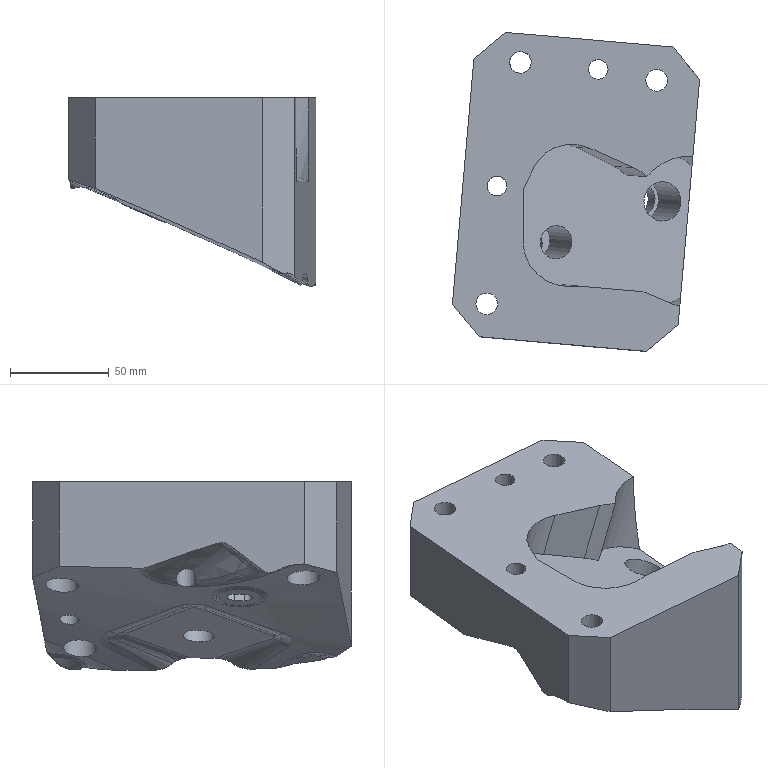Part | NX | features solid 2 | 1 solid | 91 faces | box 125.457 x 161.818 x 95.751 mm | volume 940797 mm3 | spline 50 | plane 23 | cylinder 18 | commonest cylinder face diameters 17 x4 11 x3 40 x3 8.1 x2 10 x2 16.1 x1